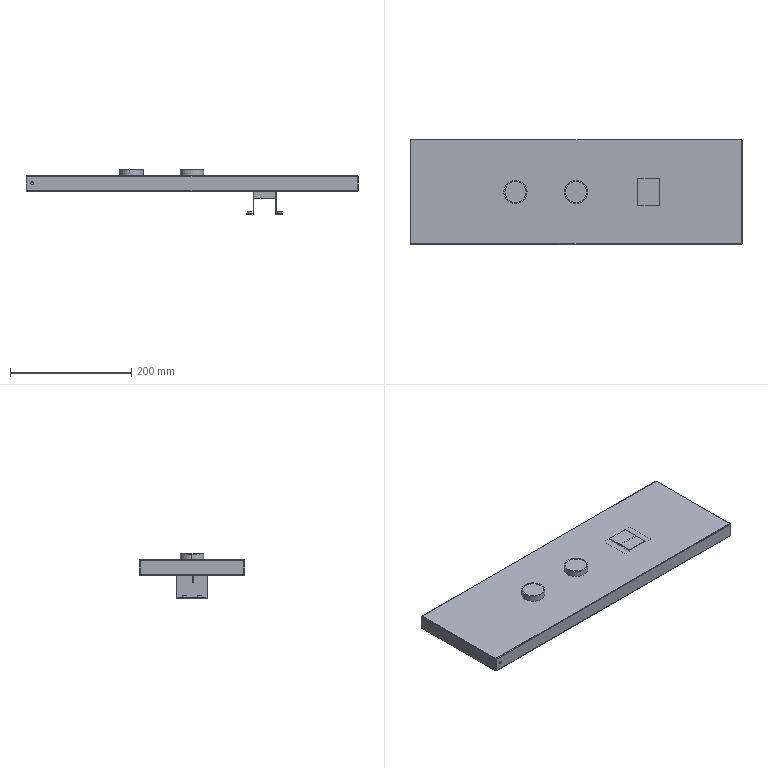Part | SolidWorks | features ICE 5, EdgeFlange 2, FlatPattern 2, SheetMetal 2, BossThin 1, CornerTrim 1, MirrorSolid 1, SMBaseFlange 1, SplitBody 1 | 4 solids | 196 faces | box 548.5 x 174 x 73 mm | volume 187457 mm3 | plane 110 | cylinder 70 | spline 16 | commonest cylinder face diameters 4.5 x18 0.2 x12 2.2 x12 3.5 x8 7.5 x8 22.3 x4